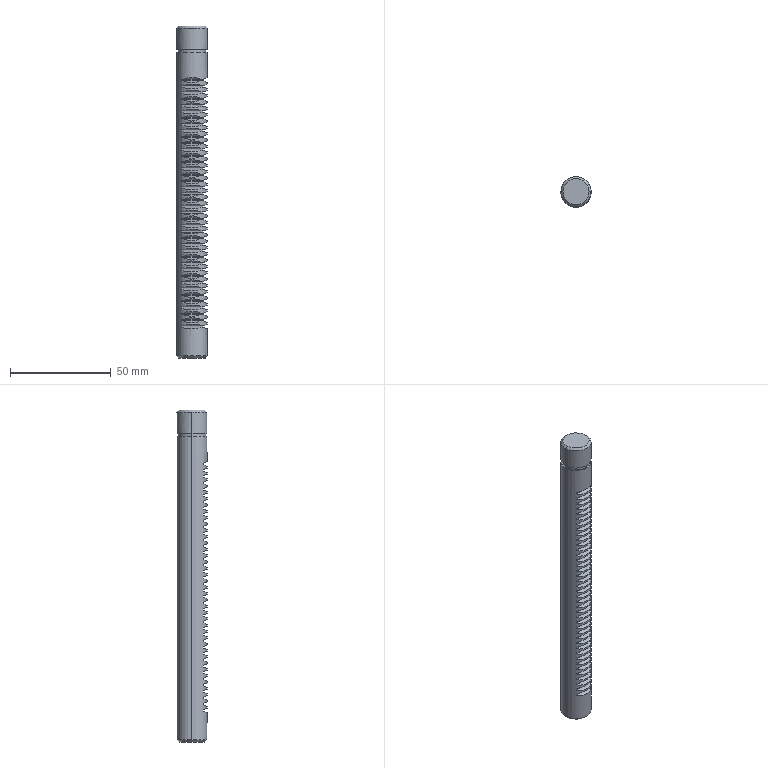Part | STEP file | Rack Gear(SP-100F).stp | 1 solid | 254 faces | box 15 x 15 x 165 mm | volume 27496 mm3 | plane 244 | cylinder 6 | cone 4 | commonest cylinder face diameters 15 x4 13.8 x2